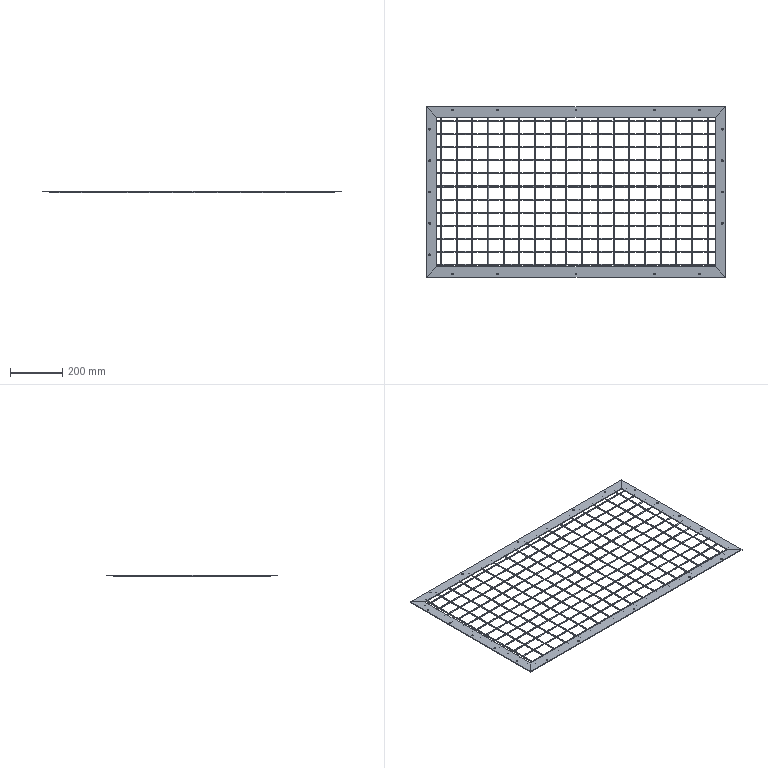Part | SolidWorks | features ICE 5, Extrusion 1, HoleWzd 1, WeldmentFeature 1 | 5 solids | 1046 faces | box 1143 x 652 x 7 mm | volume 701424 mm3 | cylinder 962 | plane 84 | commonest cylinder face diameters 4 x924 6.6 x38